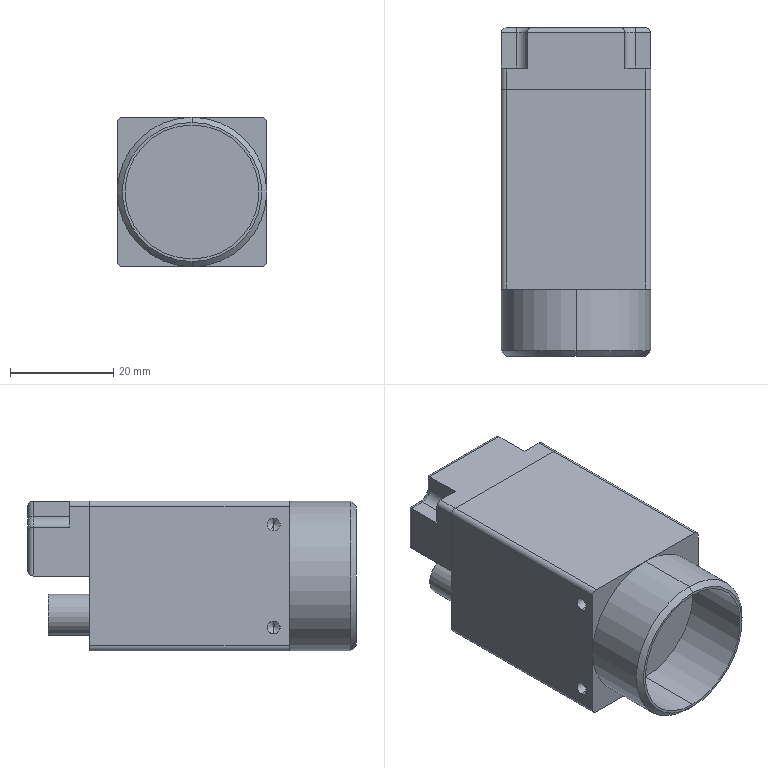Part | STEP file | MVC1000MF-M00 camera | 3 solids | 106 faces | box 29 x 63.7 x 29 mm | volume 38507 mm3 | cylinder 56 | plane 36 | cone 10 | torus 4 | commonest cylinder face diameters 2 x16 1.131 x12 2.5 x12 1 x4 6 x4 4 x2